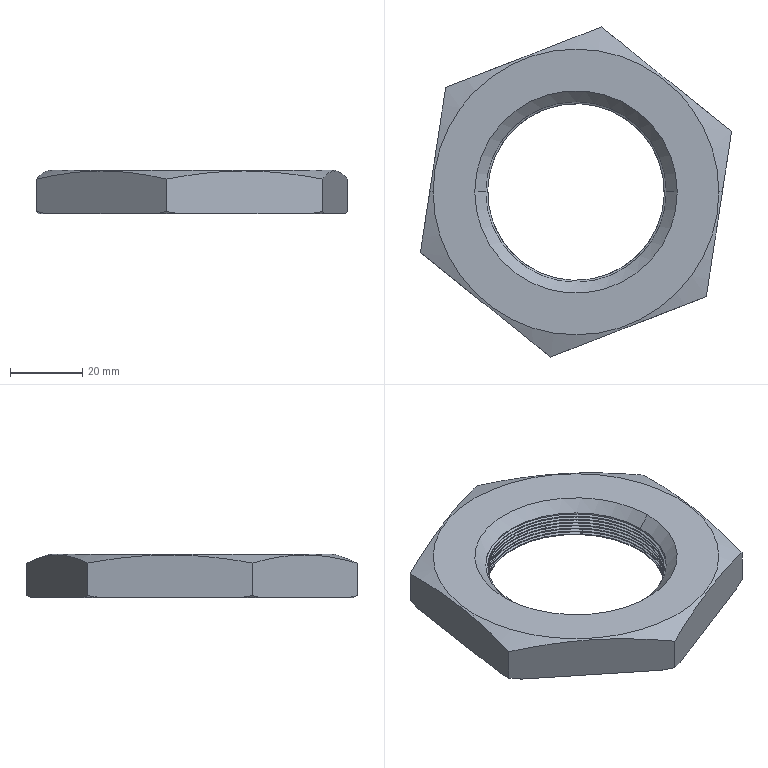Part | STEP file | Lock nut | 1 solid | 42 faces | box 86.085 x 91.305 x 12 mm | volume 41343 mm3 | cylinder 17 | cone 12 | plane 10 | spline 3 | commonest cylinder face diameters 50 x17